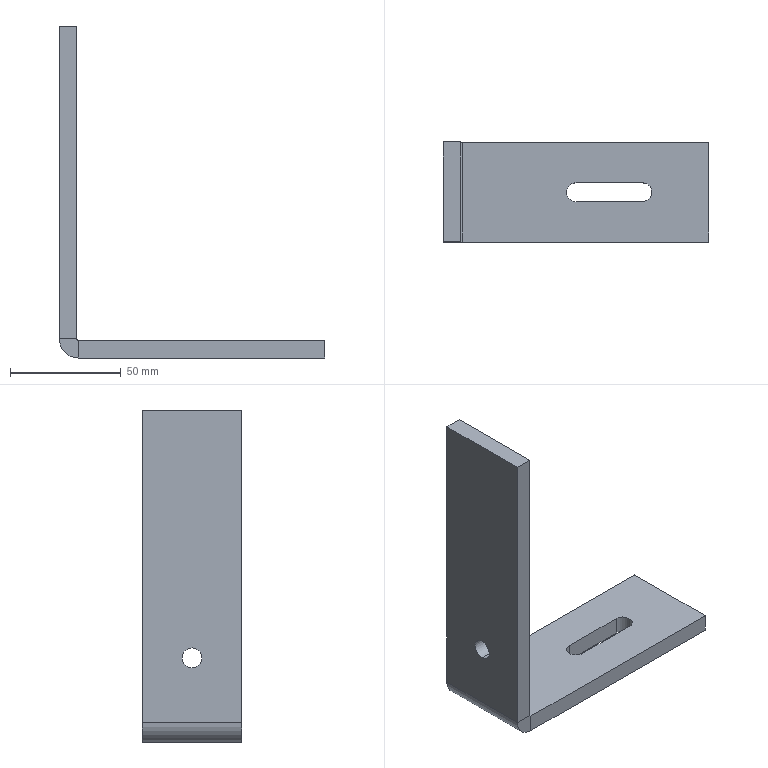Part | SolidWorks | features EdgeFlange 1, FlatPattern 1, HoleWzd 1, ICE 1, SMBaseFlange 1, SheetMetal 1 | 1 solid | 21 faces | box 120 x 45 x 150 mm | volume 90585 mm3 | plane 14 | cylinder 7 | commonest cylinder face diameters 8.5 x3 9 x2 1.473 x1 17.473 x1
STEP:
#1=CARTESIAN_POINT('',(42.788,13.156,0.));
#2=VERTEX_POINT('',#1);
#3=CARTESIAN_POINT('',(38.538,8.906,0.));
#4=VERTEX_POINT('',#3);
#5=CARTESIAN_POINT('',(42.788,8.906,0.));
#6=DIRECTION('',(0.,0.,1.));
#7=DIRECTION('',(1.,0.,0.));
#8=AXIS2_PLACEMENT_3D('',#5,#6,#7);
#9=CIRCLE('',#8,4.25);
#10=EDGE_CURVE('',#2,#4,#9,.T.);
#11=ORIENTED_EDGE('',*,*,#10,.T.);
#12=CARTESIAN_POINT('',(38.538,8.906,-8.));
#13=VERTEX_POINT('',#12);
#14=CARTESIAN_POINT('',(38.538,8.906,142.));
#15=DIRECTION('',(0.,0.,-1.));
#16=VECTOR('',#15,1000.);
#17=LINE('',#14,#16);
#18=EDGE_CURVE('',#4,#13,#17,.T.);
#19=ORIENTED_EDGE('',*,*,#18,.T.);
#20=CARTESIAN_POINT('',(42.788,13.156,-8.));
#21=VERTEX_POINT('',#20);
#22=CARTESIAN_POINT('',(42.788,8.906,-8.));
#23=DIRECTION('',(0.,0.,-1.));
#24=DIRECTION('',(-1.,0.,0.));
#25=AXIS2_PLACEMENT_3D('',#22,#23,#24);
#26=CIRCLE('',#25,4.25);
#27=EDGE_CURVE('',#13,#21,#26,.T.);
#28=ORIENTED_EDGE('',*,*,#27,.T.);
#29=CARTESIAN_POINT('',(42.788,13.156,142.));
#30=DIRECTION('',(0.,0.,-1.));
#31=VECTOR('',#30,1000.);
#32=LINE('',#29,#31);
#33=EDGE_CURVE('',#2,#21,#32,.T.);
#34=ORIENTED_EDGE('',*,*,#33,.F.);
#35=EDGE_LOOP('',(#11,#19,#28,#34));
#36=FACE_OUTER_BOUND('',#35,.T.);
#37=CARTESIAN_POINT('',(42.788,8.906,142.));
#38=DIRECTION('',(0.,0.,-1.));
#39=DIRECTION('',(-1.,0.,0.));
#40=AXIS2_PLACEMENT_3D('',#37,#38,#39);
#41=CYLINDRICAL_SURFACE('',#40,4.25);
#42=ADVANCED_FACE('',(#36),#41,.F.);
#43=CARTESIAN_POINT('',(-17.212,8.906,34.5));
#44=VERTEX_POINT('',#43);
#45=CARTESIAN_POINT('',(-17.212,8.906,25.5));
#46=VERTEX_POINT('',#45);
#47=CARTESIAN_POINT('',(-17.212,8.906,30.));
#48=DIRECTION('',(1.,0.,0.));
#49=DIRECTION('',(0.,0.,-1.));
#50=AXIS2_PLACEMENT_3D('',#47,#48,#49);
#51=CIRCLE('',#50,4.5);
#52=EDGE_CURVE('',#44,#46,#51,.T.);
#53=ORIENTED_EDGE('',*,*,#52,.F.);
#54=CARTESIAN_POINT('',(-9.212,8.906,34.5));
#55=VERTEX_POINT('',#54);
#56=CARTESIAN_POINT('',(-9.212,8.906,34.5));
#57=DIRECTION('',(1.,0.,0.));
#58=VECTOR('',#57,1000.);
#59=LINE('',#56,#58);
#60=EDGE_CURVE('',#44,#55,#59,.T.);
#61=ORIENTED_EDGE('',*,*,#60,.T.);
#62=CARTESIAN_POINT('',(-9.212,8.906,25.5));
#63=VERTEX_POINT('',#62);
#64=CARTESIAN_POINT('',(-9.212,8.906,30.));
#65=DIRECTION('',(1.,0.,0.));
#66=DIRECTION('',(0.,0.,-1.));
#67=AXIS2_PLACEMENT_3D('',#64,#65,#66);
#68=CIRCLE('',#67,4.5);
#69=EDGE_CURVE('',#55,#63,#68,.T.);
#70=ORIENTED_EDGE('',*,*,#69,.T.);
#71=CARTESIAN_POINT('',(-9.212,8.906,25.5));
#72=DIRECTION('',(1.,0.,0.));
#73=VECTOR('',#72,1000.);
#74=LINE('',#71,#73);
#75=EDGE_CURVE('',#46,#63,#74,.T.);
#76=ORIENTED_EDGE('',*,*,#75,.F.);
#77=EDGE_LOOP('',(#53,#61,#70,#76));
#78=FACE_OUTER_BOUND('',#77,.T.);
#79=CARTESIAN_POINT('',(-9.212,8.906,30.));
#80=DIRECTION('',(1.,0.,0.));
#81=DIRECTION('',(0.,0.,-1.));
#82=AXIS2_PLACEMENT_3D('',#79,#80,#81);
#83=CYLINDRICAL_SURFACE('',#82,4.5);
#84=ADVANCED_FACE('',(#78),#83,.F.);
#85=CARTESIAN_POINT('',(-8.475,-13.594,0.));
#86=VERTEX_POINT('',#85);
#87=CARTESIAN_POINT('',(102.788,-13.594,0.));
#88=VERTEX_POINT('',#87);
#89=CARTESIAN_POINT('',(-17.212,-13.594,0.));
#90=DIRECTION('',(1.,0.,0.));
#91=VECTOR('',#90,1000.);
#92=LINE('',#89,#91);
#93=EDGE_CURVE('',#86,#88,#92,.T.);
#94=ORIENTED_EDGE('',*,*,#93,.F.);
#95=CARTESIAN_POINT('',(-8.475,-13.594,-8.));
#96=VERTEX_POINT('',#95);
#97=CARTESIAN_POINT('',(-8.475,-13.594,0.));
#98=DIRECTION('',(0.,0.,-1.));
#99=VECTOR('',#98,1000.);
#100=LINE('',#97,#99);
#101=EDGE_CURVE('',#86,#96,#100,.T.);
#102=ORIENTED_EDGE('',*,*,#101,.T.);
#103=CARTESIAN_POINT('',(102.788,-13.594,-8.));
#104=VERTEX_POINT('',#103);
#105=CARTESIAN_POINT('',(-17.212,-13.594,-8.));
#106=DIRECTION('',(1.,0.,0.));
#107=VECTOR('',#106,1000.);
#108=LINE('',#105,#107);
#109=EDGE_CURVE('',#96,#104,#108,.T.);
#110=ORIENTED_EDGE('',*,*,#109,.T.);
#111=CARTESIAN_POINT('',(102.788,-13.594,-8.));
#112=DIRECTION('',(0.,0.,1.));
#113=VECTOR('',#112,1000.);
#114=LINE('',#111,#113);
#115=EDGE_CURVE('',#104,#88,#114,.T.);
#116=ORIENTED_EDGE('',*,*,#115,.T.);
#117=EDGE_LOOP('',(#94,#102,#110,#116));
#118=FACE_OUTER_BOUND('',#117,.T.);
#119=CARTESIAN_POINT('',(-17.212,-13.594,-8.));
#120=DIRECTION('',(0.,-1.,0.));
#121=DIRECTION('',(0.,0.,-1.));
#122=AXIS2_PLACEMENT_3D('',#119,#120,#121);
#123=PLANE('',#122);
#124=ADVANCED_FACE('',(#118),#123,.T.);
#125=CARTESIAN_POINT('',(72.788,4.656,-8.));
#126=VERTEX_POINT('',#125);
#127=CARTESIAN_POINT('',(42.788,4.656,-8.));
#128=VERTEX_POINT('',#127);
#129=CARTESIAN_POINT('',(72.788,4.656,-8.));
#130=DIRECTION('',(-1.,0.,0.));
#131=VECTOR('',#130,1000.);
#132=LINE('',#129,#131);
#133=EDGE_CURVE('',#126,#128,#132,.T.);
#134=ORIENTED_EDGE('',*,*,#133,.F.);
#135=CARTESIAN_POINT('',(72.788,13.156,-8.));
#136=VERTEX_POINT('',#135);
#137=CARTESIAN_POINT('',(72.788,8.906,-8.));
#138=DIRECTION('',(0.,0.,-1.));
#139=DIRECTION('',(-1.,0.,0.));
#140=AXIS2_PLACEMENT_3D('',#137,#138,#139);
#141=CIRCLE('',#140,4.25);
#142=EDGE_CURVE('',#136,#126,#141,.T.);
#143=ORIENTED_EDGE('',*,*,#142,.F.);
#144=CARTESIAN_POINT('',(72.788,13.156,-8.));
#145=DIRECTION('',(1.,0.,0.));
#146=VECTOR('',#145,1000.);
#147=LINE('',#144,#146);
#148=EDGE_CURVE('',#21,#136,#147,.T.);
#149=ORIENTED_EDGE('',*,*,#148,.F.);
#150=ORIENTED_EDGE('',*,*,#27,.F.);
#151=CARTESIAN_POINT('',(42.788,8.906,-8.));
#152=DIRECTION('',(0.,0.,-1.));
#153=DIRECTION('',(-1.,0.,0.));
#154=AXIS2_PLACEMENT_3D('',#151,#152,#153);
#155=CIRCLE('',#154,4.25);
#156=EDGE_CURVE('',#128,#13,#155,.T.);
#157=ORIENTED_EDGE('',*,*,#156,.F.);
#158=EDGE_LOOP('',(#134,#143,#149,#150,#157));
#159=FACE_BOUND('',#158,.T.);
#160=CARTESIAN_POINT('',(-8.475,31.406,-8.));
#161=VERTEX_POINT('',#160);
#162=CARTESIAN_POINT('',(-8.475,-13.594,-8.));
#163=DIRECTION('',(0.,1.,0.));
#164=VECTOR('',#163,1000.);
#165=LINE('',#162,#164);
#166=EDGE_CURVE('',#96,#161,#165,.T.);
#167=ORIENTED_EDGE('',*,*,#166,.T.);
#168=CARTESIAN_POINT('',(102.788,31.406,-8.));
#169=VERTEX_POINT('',#168);
#170=CARTESIAN_POINT('',(-17.212,31.406,-8.));
#171=DIRECTION('',(-1.,0.,0.));
#172=VECTOR('',#171,1000.);
#173=LINE('',#170,#172);
#174=EDGE_CURVE('',#169,#161,#173,.T.);
#175=ORIENTED_EDGE('',*,*,#174,.F.);
#176=CARTESIAN_POINT('',(102.788,31.406,-8.));
#177=DIRECTION('',(0.,1.,0.));
#178=VECTOR('',#177,1000.);
#179=LINE('',#176,#178);
#180=EDGE_CURVE('',#104,#169,#179,.T.);
#181=ORIENTED_EDGE('',*,*,#180,.F.);
#182=ORIENTED_EDGE('',*,*,#109,.F.);
#183=EDGE_LOOP('',(#167,#175,#181,#182));
#184=FACE_OUTER_BOUND('',#183,.T.);
#185=CARTESIAN_POINT('',(0.,0.,-8.));
#186=DIRECTION('',(0.,0.,1.));
#187=DIRECTION('',(1.,0.,0.));
#188=AXIS2_PLACEMENT_3D('',#185,#186,#187);
#189=PLANE('',#188);
#190=ADVANCED_FACE('',(#159,#184),#189,.F.);
#191=CARTESIAN_POINT('',(72.788,4.656,0.));
#192=VERTEX_POINT('',#191);
#193=CARTESIAN_POINT('',(72.788,13.156,0.));
#194=VERTEX_POINT('',#193);
#195=CARTESIAN_POINT('',(72.788,8.906,0.));
#196=DIRECTION('',(0.,0.,1.));
#197=DIRECTION('',(1.,0.,0.));
#198=AXIS2_PLACEMENT_3D('',#195,#196,#197);
#199=CIRCLE('',#198,4.25);
#200=EDGE_CURVE('',#192,#194,#199,.T.);
#201=ORIENTED_EDGE('',*,*,#200,.F.);
#202=CARTESIAN_POINT('',(42.788,4.656,0.));
#203=VERTEX_POINT('',#202);
#204=CARTESIAN_POINT('',(0.,4.656,0.));
#205=DIRECTION('',(1.,0.,0.));
#206=VECTOR('',#205,1000.);
#207=LINE('',#204,#206);
#208=EDGE_CURVE('',#203,#192,#207,.T.);
#209=ORIENTED_EDGE('',*,*,#208,.F.);
#210=CARTESIAN_POINT('',(42.788,8.906,0.));
#211=DIRECTION('',(0.,0.,1.));
#212=DIRECTION('',(1.,0.,0.));
#213=AXIS2_PLACEMENT_3D('',#210,#211,#212);
#214=CIRCLE('',#213,4.25);
#215=EDGE_CURVE('',#4,#203,#214,.T.);
#216=ORIENTED_EDGE('',*,*,#215,.F.);
#217=ORIENTED_EDGE('',*,*,#10,.F.);
#218=CARTESIAN_POINT('',(0.,13.156,0.));
#219=DIRECTION('',(-1.,0.,0.));
#220=VECTOR('',#219,1000.);
#221=LINE('',#218,#220);
#222=EDGE_CURVE('',#194,#2,#221,.T.);
#223=ORIENTED_EDGE('',*,*,#222,.F.);
#224=EDGE_LOOP('',(#201,#209,#216,#217,#223));
#225=FACE_BOUND('',#224,.T.);
#226=CARTESIAN_POINT('',(102.788,31.406,0.));
#227=VERTEX_POINT('',#226);
#228=CARTESIAN_POINT('',(-8.475,31.406,0.));
#229=VERTEX_POINT('',#228);
#230=CARTESIAN_POINT('',(-17.212,31.406,0.));
#231=DIRECTION('',(-1.,0.,0.));
#232=VECTOR('',#231,1000.);
#233=LINE('',#230,#232);
#234=EDGE_CURVE('',#227,#229,#233,.T.);
#235=ORIENTED_EDGE('',*,*,#234,.T.);
#236=CARTESIAN_POINT('',(-8.475,-13.594,0.));
#237=DIRECTION('',(0.,1.,0.));
#238=VECTOR('',#237,1000.);
#239=LINE('',#236,#238);
#240=EDGE_CURVE('',#86,#229,#239,.T.);
#241=ORIENTED_EDGE('',*,*,#240,.F.);
#242=ORIENTED_EDGE('',*,*,#93,.T.);
#243=CARTESIAN_POINT('',(102.788,31.406,0.));
#244=DIRECTION('',(0.,1.,0.));
#245=VECTOR('',#244,1000.);
#246=LINE('',#243,#245);
#247=EDGE_CURVE('',#88,#227,#246,.T.);
#248=ORIENTED_EDGE('',*,*,#247,.T.);
#249=EDGE_LOOP('',(#235,#241,#242,#248));
#250=FACE_OUTER_BOUND('',#249,.T.);
#251=CARTESIAN_POINT('',(0.,0.,0.));
#252=DIRECTION('',(0.,0.,1.));
#253=DIRECTION('',(1.,0.,0.));
#254=AXIS2_PLACEMENT_3D('',#251,#252,#253);
#255=PLANE('',#254);
#256=ADVANCED_FACE('',(#225,#250),#255,.T.);
#257=ORIENTED_EDGE('',*,*,#247,.F.);
#258=ORIENTED_EDGE('',*,*,#115,.F.);
#259=ORIENTED_EDGE('',*,*,#180,.T.);
#260=CARTESIAN_POINT('',(102.788,31.406,-8.));
#261=DIRECTION('',(0.,0.,1.));
#262=VECTOR('',#261,1000.);
#263=LINE('',#260,#262);
#264=EDGE_CURVE('',#169,#227,#263,.T.);
#265=ORIENTED_EDGE('',*,*,#264,.T.);
#266=EDGE_LOOP('',(#257,#258,#259,#265));
#267=FACE_OUTER_BOUND('',#266,.T.);
#268=CARTESIAN_POINT('',(102.788,31.406,-8.));
#269=DIRECTION('',(1.,0.,0.));
#270=DIRECTION('',(0.,1.,0.));
#271=AXIS2_PLACEMENT_3D('',#268,#269,#270);
#272=PLANE('',#271);
#273=ADVANCED_FACE('',(#267),#272,.T.);
#274=CARTESIAN_POINT('',(-8.475,31.406,0.));
#275=DIRECTION('',(0.,0.,-1.));
#276=VECTOR('',#275,1000.);
#277=LINE('',#274,#276);
#278=EDGE_CURVE('',#229,#161,#277,.T.);
#279=ORIENTED_EDGE('',*,*,#278,.F.);
#280=ORIENTED_EDGE('',*,*,#234,.F.);
#281=ORIENTED_EDGE('',*,*,#264,.F.);
#282=ORIENTED_EDGE('',*,*,#174,.T.);
#283=EDGE_LOOP('',(#279,#280,#281,#282));
#284=FACE_OUTER_BOUND('',#283,.T.);
#285=CARTESIAN_POINT('',(-17.212,31.406,-8.));
#286=DIRECTION('',(0.,1.,0.));
#287=DIRECTION('',(0.,0.,1.));
#288=AXIS2_PLACEMENT_3D('',#285,#286,#287);
#289=PLANE('',#288);
#290=ADVANCED_FACE('',(#284),#289,.T.);
#291=CARTESIAN_POINT('',(-9.212,31.406,0.7366));
#292=VERTEX_POINT('',#291);
#293=CARTESIAN_POINT('',(-17.212,31.406,0.7366));
#294=VERTEX_POINT('',#293);
#295=CARTESIAN_POINT('',(-17.212,31.406,0.7366));
#296=DIRECTION('',(-1.,0.,0.));
#297=VECTOR('',#296,1000.);
#298=LINE('',#295,#297);
#299=EDGE_CURVE('',#292,#294,#298,.T.);
#300=ORIENTED_EDGE('',*,*,#299,.F.);
#301=CARTESIAN_POINT('',(-8.475,31.406,0.7366));
#302=DIRECTION('',(0.,1.,0.));
#303=DIRECTION('',(0.,0.,-1.));
#304=AXIS2_PLACEMENT_3D('',#301,#302,#303);
#305=CIRCLE('',#304,0.7366);
#306=EDGE_CURVE('',#229,#292,#305,.T.);
#307=ORIENTED_EDGE('',*,*,#306,.F.);
#308=ORIENTED_EDGE('',*,*,#278,.T.);
#309=CARTESIAN_POINT('',(-8.475,31.406,0.7366));
#310=DIRECTION('',(0.,1.,0.));
#311=DIRECTION('',(0.,0.,-1.));
#312=AXIS2_PLACEMENT_3D('',#309,#310,#311);
#313=CIRCLE('',#312,8.737);
#314=EDGE_CURVE('',#161,#294,#313,.T.);
#315=ORIENTED_EDGE('',*,*,#314,.T.);
#316=EDGE_LOOP('',(#300,#307,#308,#315));
#317=FACE_OUTER_BOUND('',#316,.T.);
#318=CARTESIAN_POINT('',(-8.475,31.406,0.7366));
#319=DIRECTION('',(0.,1.,0.));
#320=DIRECTION('',(0.,0.,1.));
#321=AXIS2_PLACEMENT_3D('',#318,#319,#320);
#322=PLANE('',#321);
#323=ADVANCED_FACE('',(#317),#322,.T.);
#324=CARTESIAN_POINT('',(-9.212,-13.594,0.7366));
#325=VERTEX_POINT('',#324);
#326=CARTESIAN_POINT('',(-8.475,-13.594,0.7366));
#327=DIRECTION('',(0.,-1.,0.));
#328=DIRECTION('',(0.,0.,-1.));
#329=AXIS2_PLACEMENT_3D('',#326,#327,#328);
#330=CIRCLE('',#329,0.7366);
#331=EDGE_CURVE('',#325,#86,#330,.T.);
#332=ORIENTED_EDGE('',*,*,#331,.F.);
#333=CARTESIAN_POINT('',(-17.212,-13.594,0.7366));
#334=VERTEX_POINT('',#333);
#335=CARTESIAN_POINT('',(-9.212,-13.594,0.7366));
#336=DIRECTION('',(-1.,0.,0.));
#337=VECTOR('',#336,1000.);
#338=LINE('',#335,#337);
#339=EDGE_CURVE('',#325,#334,#338,.T.);
#340=ORIENTED_EDGE('',*,*,#339,.T.);
#341=CARTESIAN_POINT('',(-8.475,-13.594,0.7366));
#342=DIRECTION('',(0.,-1.,0.));
#343=DIRECTION('',(0.,0.,-1.));
#344=AXIS2_PLACEMENT_3D('',#341,#342,#343);
#345=CIRCLE('',#344,8.737);
#346=EDGE_CURVE('',#334,#96,#345,.T.);
#347=ORIENTED_EDGE('',*,*,#346,.T.);
#348=ORIENTED_EDGE('',*,*,#101,.F.);
#349=EDGE_LOOP('',(#332,#340,#347,#348));
#350=FACE_OUTER_BOUND('',#349,.T.);
#351=CARTESIAN_POINT('',(-8.475,-13.594,0.7366));
#352=DIRECTION('',(0.,1.,0.));
#353=DIRECTION('',(0.,0.,1.));
#354=AXIS2_PLACEMENT_3D('',#351,#352,#353);
#355=PLANE('',#354);
#356=ADVANCED_FACE('',(#350),#355,.F.);
#357=ORIENTED_EDGE('',*,*,#166,.F.);
#358=ORIENTED_EDGE('',*,*,#346,.F.);
#359=CARTESIAN_POINT('',(-17.212,31.406,0.7366));
#360=DIRECTION('',(0.,1.,0.));
#361=VECTOR('',#360,1000.);
#362=LINE('',#359,#361);
#363=EDGE_CURVE('',#334,#294,#362,.T.);
#364=ORIENTED_EDGE('',*,*,#363,.T.);
#365=ORIENTED_EDGE('',*,*,#314,.F.);
#366=EDGE_LOOP('',(#357,#358,#364,#365));
#367=FACE_OUTER_BOUND('',#366,.T.);
#368=CARTESIAN_POINT('',(-8.475,-13.594,0.7366));
#369=DIRECTION('',(0.,-1.,0.));
#370=DIRECTION('',(-1.,0.,0.));
#371=AXIS2_PLACEMENT_3D('',#368,#369,#370);
#372=CYLINDRICAL_SURFACE('',#371,8.737);
#373=ADVANCED_FACE('',(#367),#372,.T.);
#374=ORIENTED_EDGE('',*,*,#240,.T.);
#375=ORIENTED_EDGE('',*,*,#306,.T.);
#376=CARTESIAN_POINT('',(-9.212,31.406,0.7366));
#377=DIRECTION('',(0.,-1.,0.));
#378=VECTOR('',#377,1000.);
#379=LINE('',#376,#378);
#380=EDGE_CURVE('',#292,#325,#379,.T.);
#381=ORIENTED_EDGE('',*,*,#380,.T.);
#382=ORIENTED_EDGE('',*,*,#331,.T.);
#383=EDGE_LOOP('',(#374,#375,#381,#382));
#384=FACE_OUTER_BOUND('',#383,.T.);
#385=CARTESIAN_POINT('',(-8.475,-13.594,0.7366));
#386=DIRECTION('',(0.,-1.,0.));
#387=DIRECTION('',(-1.,0.,0.));
#388=AXIS2_PLACEMENT_3D('',#385,#386,#387);
#389=CYLINDRICAL_SURFACE('',#388,0.7366);
#390=ADVANCED_FACE('',(#384),#389,.F.);
#391=ORIENTED_EDGE('',*,*,#299,.T.);
#392=CARTESIAN_POINT('',(-17.212,31.406,142.));
#393=VERTEX_POINT('',#392);
#394=CARTESIAN_POINT('',(-17.212,31.406,0.));
#395=DIRECTION('',(0.,0.,-1.));
#396=VECTOR('',#395,1000.);
#397=LINE('',#394,#396);
#398=EDGE_CURVE('',#393,#294,#397,.T.);
#399=ORIENTED_EDGE('',*,*,#398,.F.);
#400=CARTESIAN_POINT('',(-9.212,31.406,142.));
#401=VERTEX_POINT('',#400);
#402=CARTESIAN_POINT('',(-17.212,31.406,142.));
#403=DIRECTION('',(1.,0.,0.));
#404=VECTOR('',#403,1000.);
#405=LINE('',#402,#404);
#406=EDGE_CURVE('',#393,#401,#405,.T.);
#407=ORIENTED_EDGE('',*,*,#406,.T.);
#408=CARTESIAN_POINT('',(-9.212,31.406,0.));
#409=DIRECTION('',(0.,0.,-1.));
#410=VECTOR('',#409,1000.);
#411=LINE('',#408,#410);
#412=EDGE_CURVE('',#401,#292,#411,.T.);
#413=ORIENTED_EDGE('',*,*,#412,.T.);
#414=EDGE_LOOP('',(#391,#399,#407,#413));
#415=FACE_OUTER_BOUND('',#414,.T.);
#416=CARTESIAN_POINT('',(-17.212,31.406,0.));
#417=DIRECTION('',(0.,-1.,0.));
#418=DIRECTION('',(0.,0.,-1.));
#419=AXIS2_PLACEMENT_3D('',#416,#417,#418);
#420=PLANE('',#419);
#421=ADVANCED_FACE('',(#415),#420,.F.);
#422=ORIENTED_EDGE('',*,*,#339,.F.);
#423=CARTESIAN_POINT('',(-9.212,-13.594,142.));
#424=VERTEX_POINT('',#423);
#425=CARTESIAN_POINT('',(-9.212,-13.594,142.));
#426=DIRECTION('',(0.,0.,1.));
#427=VECTOR('',#426,1000.);
#428=LINE('',#425,#427);
#429=EDGE_CURVE('',#325,#424,#428,.T.);
#430=ORIENTED_EDGE('',*,*,#429,.T.);
#431=CARTESIAN_POINT('',(-17.212,-13.594,142.));
#432=VERTEX_POINT('',#431);
#433=CARTESIAN_POINT('',(-17.212,-13.594,142.));
#434=DIRECTION('',(1.,0.,0.));
#435=VECTOR('',#434,1000.);
#436=LINE('',#433,#435);
#437=EDGE_CURVE('',#432,#424,#436,.T.);
#438=ORIENTED_EDGE('',*,*,#437,.F.);
#439=CARTESIAN_POINT('',(-17.212,-13.594,0.));
#440=DIRECTION('',(0.,0.,1.));
#441=VECTOR('',#440,1000.);
#442=LINE('',#439,#441);
#443=EDGE_CURVE('',#334,#432,#442,.T.);
#444=ORIENTED_EDGE('',*,*,#443,.F.);
#445=EDGE_LOOP('',(#422,#430,#438,#444));
#446=FACE_OUTER_BOUND('',#445,.T.);
#447=CARTESIAN_POINT('',(-17.212,-13.594,142.));
#448=DIRECTION('',(0.,1.,0.));
#449=DIRECTION('',(0.,0.,1.));
#450=AXIS2_PLACEMENT_3D('',#447,#448,#449);
#451=PLANE('',#450);
#452=ADVANCED_FACE('',(#446),#451,.F.);
#453=CARTESIAN_POINT('',(-17.212,8.906,30.));
#454=DIRECTION('',(1.,0.,0.));
#455=DIRECTION('',(0.,0.,-1.));
#456=AXIS2_PLACEMENT_3D('',#453,#454,#455);
#457=CIRCLE('',#456,4.5);
#458=EDGE_CURVE('',#46,#44,#457,.T.);
#459=ORIENTED_EDGE('',*,*,#458,.T.);
#460=ORIENTED_EDGE('',*,*,#52,.T.);
#461=EDGE_LOOP('',(#459,#460));
#462=FACE_BOUND('',#461,.T.);
#463=ORIENTED_EDGE('',*,*,#363,.F.);
#464=ORIENTED_EDGE('',*,*,#443,.T.);
#465=CARTESIAN_POINT('',(-17.212,0.,142.));
#466=DIRECTION('',(0.,1.,0.));
#467=VECTOR('',#466,1000.);
#468=LINE('',#465,#467);
#469=EDGE_CURVE('',#432,#393,#468,.T.);
#470=ORIENTED_EDGE('',*,*,#469,.T.);
#471=ORIENTED_EDGE('',*,*,#398,.T.);
#472=EDGE_LOOP('',(#463,#464,#470,#471));
#473=FACE_OUTER_BOUND('',#472,.T.);
#474=CARTESIAN_POINT('',(-17.212,0.,0.));
#475=DIRECTION('',(1.,0.,0.));
#476=DIRECTION('',(0.,0.,-1.));
#477=AXIS2_PLACEMENT_3D('',#474,#475,#476);
#478=PLANE('',#477);
#479=ADVANCED_FACE('',(#462,#473),#478,.F.);
#480=CARTESIAN_POINT('',(-9.212,8.906,30.));
#481=DIRECTION('',(1.,0.,0.));
#482=DIRECTION('',(0.,0.,-1.));
#483=AXIS2_PLACEMENT_3D('',#480,#481,#482);
#484=CIRCLE('',#483,4.5);
#485=EDGE_CURVE('',#63,#55,#484,.T.);
#486=ORIENTED_EDGE('',*,*,#485,.F.);
#487=ORIENTED_EDGE('',*,*,#69,.F.);
#488=EDGE_LOOP('',(#486,#487));
#489=FACE_BOUND('',#488,.T.);
#490=ORIENTED_EDGE('',*,*,#429,.F.);
#491=ORIENTED_EDGE('',*,*,#380,.F.);
#492=ORIENTED_EDGE('',*,*,#412,.F.);
#493=CARTESIAN_POINT('',(-9.212,31.406,142.));
#494=DIRECTION('',(0.,1.,0.));
#495=VECTOR('',#494,1000.);
#496=LINE('',#493,#495);
#497=EDGE_CURVE('',#424,#401,#496,.T.);
#498=ORIENTED_EDGE('',*,*,#497,.F.);
#499=EDGE_LOOP('',(#490,#491,#492,#498));
#500=FACE_OUTER_BOUND('',#499,.T.);
#501=CARTESIAN_POINT('',(-9.212,0.,0.));
#502=DIRECTION('',(1.,0.,0.));
#503=DIRECTION('',(0.,0.,-1.));
#504=AXIS2_PLACEMENT_3D('',#501,#502,#503);
#505=PLANE('',#504);
#506=ADVANCED_FACE('',(#489,#500),#505,.T.);
#507=ORIENTED_EDGE('',*,*,#497,.T.);
#508=ORIENTED_EDGE('',*,*,#406,.F.);
#509=ORIENTED_EDGE('',*,*,#469,.F.);
#510=ORIENTED_EDGE('',*,*,#437,.T.);
#511=EDGE_LOOP('',(#507,#508,#509,#510));
#512=FACE_OUTER_BOUND('',#511,.T.);
#513=CARTESIAN_POINT('',(-17.212,31.406,142.));
#514=DIRECTION('',(0.,0.,-1.));
#515=DIRECTION('',(-1.,0.,0.));
#516=AXIS2_PLACEMENT_3D('',#513,#514,#515);
#517=PLANE('',#516);
#518=ADVANCED_FACE('',(#512),#517,.F.);
#519=ORIENTED_EDGE('',*,*,#60,.F.);
#520=ORIENTED_EDGE('',*,*,#458,.F.);
#521=ORIENTED_EDGE('',*,*,#75,.T.);
#522=ORIENTED_EDGE('',*,*,#485,.T.);
#523=EDGE_LOOP('',(#519,#520,#521,#522));
#524=FACE_OUTER_BOUND('',#523,.T.);
#525=CARTESIAN_POINT('',(-9.212,8.906,30.));
#526=DIRECTION('',(1.,0.,0.));
#527=DIRECTION('',(0.,0.,-1.));
#528=AXIS2_PLACEMENT_3D('',#525,#526,#527);
#529=CYLINDRICAL_SURFACE('',#528,4.5);
#530=ADVANCED_FACE('',(#524),#529,.F.);
#531=ORIENTED_EDGE('',*,*,#200,.T.);
#532=CARTESIAN_POINT('',(72.788,13.156,142.));
#533=DIRECTION('',(0.,0.,-1.));
#534=VECTOR('',#533,1000.);
#535=LINE('',#532,#534);
#536=EDGE_CURVE('',#194,#136,#535,.T.);
#537=ORIENTED_EDGE('',*,*,#536,.T.);
#538=ORIENTED_EDGE('',*,*,#142,.T.);
#539=CARTESIAN_POINT('',(72.788,4.656,142.));
#540=DIRECTION('',(0.,0.,-1.));
#541=VECTOR('',#540,1000.);
#542=LINE('',#539,#541);
#543=EDGE_CURVE('',#192,#126,#542,.T.);
#544=ORIENTED_EDGE('',*,*,#543,.F.);
#545=EDGE_LOOP('',(#531,#537,#538,#544));
#546=FACE_OUTER_BOUND('',#545,.T.);
#547=CARTESIAN_POINT('',(72.788,8.906,142.));
#548=DIRECTION('',(0.,0.,-1.));
#549=DIRECTION('',(-1.,0.,0.));
#550=AXIS2_PLACEMENT_3D('',#547,#548,#549);
#551=CYLINDRICAL_SURFACE('',#550,4.25);
#552=ADVANCED_FACE('',(#546),#551,.F.);
#553=ORIENTED_EDGE('',*,*,#222,.T.);
#554=ORIENTED_EDGE('',*,*,#33,.T.);
#555=ORIENTED_EDGE('',*,*,#148,.T.);
#556=ORIENTED_EDGE('',*,*,#536,.F.);
#557=EDGE_LOOP('',(#553,#554,#555,#556));
#558=FACE_OUTER_BOUND('',#557,.T.);
#559=CARTESIAN_POINT('',(72.788,13.156,142.));
#560=DIRECTION('',(0.,1.,0.));
#561=DIRECTION('',(0.,0.,1.));
#562=AXIS2_PLACEMENT_3D('',#559,#560,#561);
#563=PLANE('',#562);
#564=ADVANCED_FACE('',(#558),#563,.F.);
#565=ORIENTED_EDGE('',*,*,#18,.F.);
#566=ORIENTED_EDGE('',*,*,#215,.T.);
#567=CARTESIAN_POINT('',(42.788,4.656,142.));
#568=DIRECTION('',(0.,0.,-1.));
#569=VECTOR('',#568,1000.);
#570=LINE('',#567,#569);
#571=EDGE_CURVE('',#203,#128,#570,.T.);
#572=ORIENTED_EDGE('',*,*,#571,.T.);
#573=ORIENTED_EDGE('',*,*,#156,.T.);
#574=EDGE_LOOP('',(#565,#566,#572,#573));
#575=FACE_OUTER_BOUND('',#574,.T.);
#576=CARTESIAN_POINT('',(42.788,8.906,142.));
#577=DIRECTION('',(0.,0.,-1.));
#578=DIRECTION('',(-1.,0.,0.));
#579=AXIS2_PLACEMENT_3D('',#576,#577,#578);
#580=CYLINDRICAL_SURFACE('',#579,4.25);
#581=ADVANCED_FACE('',(#575),#580,.F.);
#582=ORIENTED_EDGE('',*,*,#208,.T.);
#583=ORIENTED_EDGE('',*,*,#543,.T.);
#584=ORIENTED_EDGE('',*,*,#133,.T.);
#585=ORIENTED_EDGE('',*,*,#571,.F.);
#586=EDGE_LOOP('',(#582,#583,#584,#585));
#587=FACE_OUTER_BOUND('',#586,.T.);
#588=CARTESIAN_POINT('',(72.788,4.656,142.));
#589=DIRECTION('',(0.,-1.,0.));
#590=DIRECTION('',(0.,0.,-1.));
#591=AXIS2_PLACEMENT_3D('',#588,#589,#590);
#592=PLANE('',#591);
#593=ADVANCED_FACE('',(#587),#592,.F.);
#594=CLOSED_SHELL('',(#42,#84,#124,#190,#256,#273,#290,#323,#356,#373,#390,#421,#452,#479,#506,#518,#530,#552,#564,#581,#593));
#595=MANIFOLD_SOLID_BREP('',#594);
#596=CARTESIAN_POINT('',(0.,0.,0.));
#597=DIRECTION('',(0.,0.,1.));
#598=DIRECTION('',(1.,0.,0.));
#599=AXIS2_PLACEMENT_3D('',#596,#597,#598);
#600=(LENGTH_UNIT()NAMED_UNIT(*)SI_UNIT(.MILLI.,.METRE.));
#601=UNCERTAINTY_MEASURE_WITH_UNIT(LENGTH_MEASURE(0.00001),#600,'','');
#602=(NAMED_UNIT(*)PLANE_ANGLE_UNIT()SI_UNIT($,.RADIAN.));
#603=(NAMED_UNIT(*)SI_UNIT($,.STERADIAN.)SOLID_ANGLE_UNIT());
#604=(GEOMETRIC_REPRESENTATION_CONTEXT(3)GLOBAL_UNCERTAINTY_ASSIGNED_CONTEXT((#601))GLOBAL_UNIT_ASSIGNED_CONTEXT((#600,#602,#603))REPRESENTATION_CONTEXT('',''));
#605=ADVANCED_BREP_SHAPE_REPRESENTATION('',(#595,#599),#604);